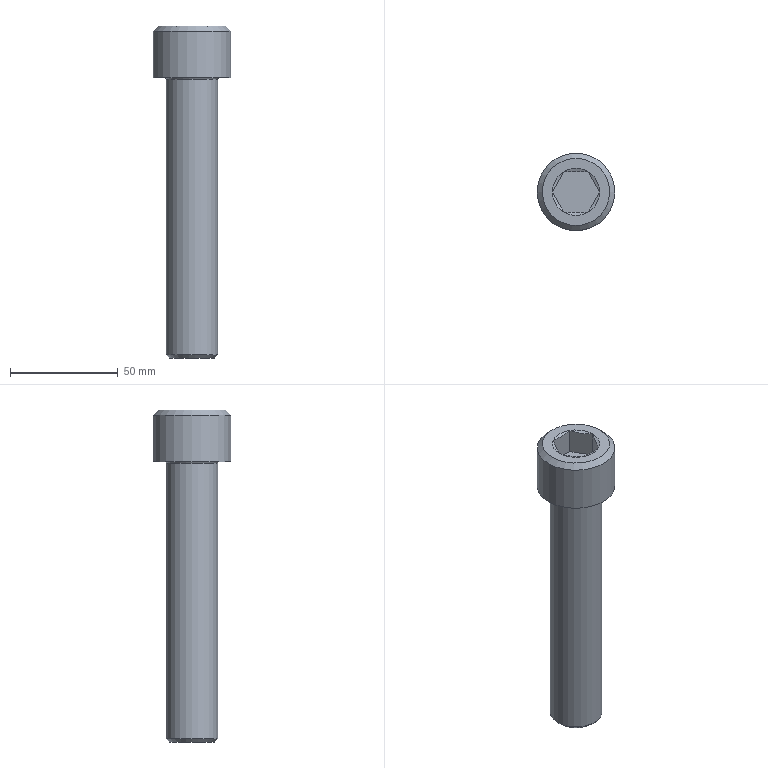Part | STEP file | solid 138 | 1 solid | 21 faces | box 36 x 36 x 154 mm | volume 79089 mm3 | plane 10 | sphere 6 | cylinder 2 | cone 2 | torus 1 | commonest cylinder face diameters 24 x1 36 x1